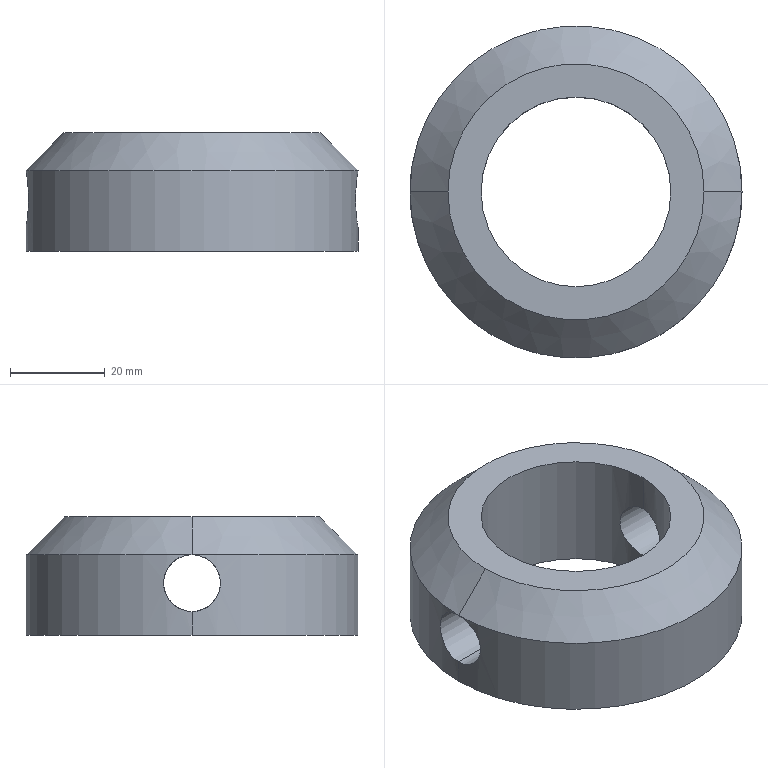Part | SolidWorks | features Chamfer 1, Extrusion 1, ICE 1 | 1 solid | 12 faces | box 70 x 70 x 25 mm | volume 54879 mm3 | cylinder 8 | cone 2 | plane 2 | commonest cylinder face diameters 12 x4 40 x2 70 x2
STEP:
#1=CARTESIAN_POINT('',(-35.,0.,17.));
#2=VERTEX_POINT('',#1);
#3=CARTESIAN_POINT('',(-35.,0.,5.));
#4=VERTEX_POINT('',#3);
#5=CARTESIAN_POINT('',(-35.,0.,17.));
#6=CARTESIAN_POINT('',(-35.,-0.3971,17.));
#7=CARTESIAN_POINT('',(-34.993,-0.7875,16.961));
#8=CARTESIAN_POINT('',(-34.974,-1.363,16.846));
#9=CARTESIAN_POINT('',(-34.966,-1.554,16.799));
#10=CARTESIAN_POINT('',(-34.947,-1.931,16.684));
#11=CARTESIAN_POINT('',(-34.936,-2.118,16.617));
#12=CARTESIAN_POINT('',(-34.9,-2.663,16.391));
#13=CARTESIAN_POINT('',(-34.872,-3.007,16.207));
#14=CARTESIAN_POINT('',(-34.81,-3.659,15.772));
#15=CARTESIAN_POINT('',(-34.776,-3.967,15.519));
#16=CARTESIAN_POINT('',(-34.708,-4.519,14.966));
#17=CARTESIAN_POINT('',(-34.675,-4.767,14.665));
#18=CARTESIAN_POINT('',(-34.611,-5.206,14.009));
#19=CARTESIAN_POINT('',(-34.583,-5.392,13.661));
#20=CARTESIAN_POINT('',(-34.547,-5.616,13.12));
#21=CARTESIAN_POINT('',(-34.536,-5.682,12.936));
#22=CARTESIAN_POINT('',(-34.517,-5.797,12.56));
#23=CARTESIAN_POINT('',(-34.508,-5.845,12.367));
#24=CARTESIAN_POINT('',(-34.489,-5.961,11.786));
#25=CARTESIAN_POINT('',(-34.482,-6.,11.397));
#26=CARTESIAN_POINT('',(-34.482,-6.,10.613));
#27=CARTESIAN_POINT('',(-34.489,-5.961,10.214));
#28=CARTESIAN_POINT('',(-34.515,-5.808,9.444));
#29=CARTESIAN_POINT('',(-34.534,-5.695,9.07));
#30=CARTESIAN_POINT('',(-34.57,-5.469,8.524));
#31=CARTESIAN_POINT('',(-34.584,-5.384,8.345));
#32=CARTESIAN_POINT('',(-34.612,-5.199,7.998));
#33=CARTESIAN_POINT('',(-34.627,-5.098,7.83));
#34=CARTESIAN_POINT('',(-34.674,-4.773,7.343));
#35=CARTESIAN_POINT('',(-34.707,-4.524,7.039));
#36=CARTESIAN_POINT('',(-34.776,-3.966,6.48));
#37=CARTESIAN_POINT('',(-34.809,-3.664,6.233));
#38=CARTESIAN_POINT('',(-34.856,-3.177,5.907));
#39=CARTESIAN_POINT('',(-34.871,-3.01,5.806));
#40=CARTESIAN_POINT('',(-34.899,-2.662,5.619));
#41=CARTESIAN_POINT('',(-34.912,-2.483,5.534));
#42=CARTESIAN_POINT('',(-34.948,-1.939,5.308));
#43=CARTESIAN_POINT('',(-34.967,-1.565,5.194));
#44=CARTESIAN_POINT('',(-34.993,-0.7947,5.04));
#45=CARTESIAN_POINT('',(-35.,-0.3971,5.));
#46=CARTESIAN_POINT('',(-35.,0.,5.));
#47=B_SPLINE_CURVE_WITH_KNOTS('',3,(#5,#6,#7,#8,#9,#10,#11,#12,#13,#14,#15,#16,#17,#18,#19,#20,#21,#22,#23,#24,#25,#26,#27,#28,#29,#30,#31,#32,#33,#34,#35,#36,#37,#38,#39,#40,#41,#42,#43,#44,#45,#46),.UNSPECIFIED.,.F.,.F.,(4,2,2,2,2,2,2,2,2,2,2,2,2,2,2,2,2,2,2,2,4),(0.01879,0.01996,0.02055,0.02114,0.02231,0.02349,0.02466,0.02583,0.02642,0.02701,0.02818,0.02936,0.03053,0.03112,0.03171,0.03288,0.03405,0.03464,0.03523,0.0364,0.03758),.UNSPECIFIED.);
#48=EDGE_CURVE('',#2,#4,#47,.T.);
#49=ORIENTED_EDGE('',*,*,#48,.F.);
#50=CARTESIAN_POINT('',(-20.,0.,17.));
#51=VERTEX_POINT('',#50);
#52=CARTESIAN_POINT('',(-35.,0.,17.));
#53=DIRECTION('',(1.,0.,0.));
#54=VECTOR('',#53,1000.);
#55=LINE('',#52,#54);
#56=EDGE_CURVE('',#2,#51,#55,.T.);
#57=ORIENTED_EDGE('',*,*,#56,.T.);
#58=CARTESIAN_POINT('',(-20.,0.,5.));
#59=VERTEX_POINT('',#58);
#60=CARTESIAN_POINT('',(-20.,0.,17.));
#61=CARTESIAN_POINT('',(-20.,-0.3989,17.));
#62=CARTESIAN_POINT('',(-19.988,-0.7907,16.961));
#63=CARTESIAN_POINT('',(-19.954,-1.368,16.845));
#64=CARTESIAN_POINT('',(-19.94,-1.559,16.797));
#65=CARTESIAN_POINT('',(-19.907,-1.937,16.682));
#66=CARTESIAN_POINT('',(-19.888,-2.125,16.615));
#67=CARTESIAN_POINT('',(-19.824,-2.669,16.388));
#68=CARTESIAN_POINT('',(-19.775,-3.013,16.204));
#69=CARTESIAN_POINT('',(-19.692,-3.501,15.877));
#70=CARTESIAN_POINT('',(-19.663,-3.659,15.759));
#71=CARTESIAN_POINT('',(-19.604,-3.962,15.51));
#72=CARTESIAN_POINT('',(-19.574,-4.107,15.379));
#73=CARTESIAN_POINT('',(-19.485,-4.519,14.966));
#74=CARTESIAN_POINT('',(-19.425,-4.767,14.665));
#75=CARTESIAN_POINT('',(-19.312,-5.205,14.01));
#76=CARTESIAN_POINT('',(-19.261,-5.39,13.665));
#77=CARTESIAN_POINT('',(-19.196,-5.615,13.124));
#78=CARTESIAN_POINT('',(-19.176,-5.681,12.94));
#79=CARTESIAN_POINT('',(-19.142,-5.796,12.563));
#80=CARTESIAN_POINT('',(-19.127,-5.845,12.369));
#81=CARTESIAN_POINT('',(-19.091,-5.961,11.788));
#82=CARTESIAN_POINT('',(-19.079,-6.,11.397));
#83=CARTESIAN_POINT('',(-19.079,-6.,10.609));
#84=CARTESIAN_POINT('',(-19.091,-5.961,10.209));
#85=CARTESIAN_POINT('',(-19.139,-5.806,9.437));
#86=CARTESIAN_POINT('',(-19.174,-5.692,9.062));
#87=CARTESIAN_POINT('',(-19.261,-5.389,8.333));
#88=CARTESIAN_POINT('',(-19.313,-5.202,7.985));
#89=CARTESIAN_POINT('',(-19.397,-4.877,7.5));
#90=CARTESIAN_POINT('',(-19.425,-4.761,7.343));
#91=CARTESIAN_POINT('',(-19.485,-4.513,7.041));
#92=CARTESIAN_POINT('',(-19.515,-4.38,6.894));
#93=CARTESIAN_POINT('',(-19.605,-3.964,6.479));
#94=CARTESIAN_POINT('',(-19.664,-3.664,6.232));
#95=CARTESIAN_POINT('',(-19.774,-3.015,5.798));
#96=CARTESIAN_POINT('',(-19.825,-2.664,5.61));
#97=CARTESIAN_POINT('',(-19.909,-1.941,5.309));
#98=CARTESIAN_POINT('',(-19.942,-1.566,5.195));
#99=CARTESIAN_POINT('',(-19.977,-0.985,5.078));
#100=CARTESIAN_POINT('',(-19.985,-0.787,5.049));
#101=CARTESIAN_POINT('',(-19.997,-0.3932,5.01));
#102=CARTESIAN_POINT('',(-20.,-0.1965,5.));
#103=CARTESIAN_POINT('',(-20.,0.,5.));
#104=B_SPLINE_CURVE_WITH_KNOTS('',3,(#60,#61,#62,#63,#64,#65,#66,#67,#68,#69,#70,#71,#72,#73,#74,#75,#76,#77,#78,#79,#80,#81,#82,#83,#84,#85,#86,#87,#88,#89,#90,#91,#92,#93,#94,#95,#96,#97,#98,#99,#100,#101,#102,#103),.UNSPECIFIED.,.F.,.F.,(4,2,2,2,2,2,2,2,2,2,2,2,2,2,2,2,2,2,2,2,2,4),(0.,0.001179,0.001769,0.002359,0.003538,0.004127,0.004717,0.005896,0.007076,0.007665,0.008255,0.009434,0.01061,0.01179,0.01297,0.01356,0.01415,0.01533,0.01651,0.01769,0.01828,0.01887),.UNSPECIFIED.);
#105=EDGE_CURVE('',#51,#59,#104,.T.);
#106=ORIENTED_EDGE('',*,*,#105,.T.);
#107=CARTESIAN_POINT('',(-35.,0.,5.));
#108=DIRECTION('',(1.,0.,0.));
#109=VECTOR('',#108,1000.);
#110=LINE('',#107,#109);
#111=EDGE_CURVE('',#4,#59,#110,.T.);
#112=ORIENTED_EDGE('',*,*,#111,.F.);
#113=EDGE_LOOP('',(#49,#57,#106,#112));
#114=FACE_OUTER_BOUND('',#113,.T.);
#115=CARTESIAN_POINT('',(-35.,0.,11.));
#116=DIRECTION('',(1.,0.,0.));
#117=DIRECTION('',(0.,0.,-1.));
#118=AXIS2_PLACEMENT_3D('',#115,#116,#117);
#119=CYLINDRICAL_SURFACE('',#118,6.);
#120=ADVANCED_FACE('',(#114),#119,.F.);
#121=CARTESIAN_POINT('',(20.,0.,5.));
#122=VERTEX_POINT('',#121);
#123=CARTESIAN_POINT('',(20.,0.,17.));
#124=VERTEX_POINT('',#123);
#125=CARTESIAN_POINT('',(20.,0.,5.));
#126=CARTESIAN_POINT('',(20.,-0.3989,5.));
#127=CARTESIAN_POINT('',(19.988,-0.7907,5.039));
#128=CARTESIAN_POINT('',(19.954,-1.368,5.155));
#129=CARTESIAN_POINT('',(19.94,-1.559,5.203));
#130=CARTESIAN_POINT('',(19.907,-1.937,5.318));
#131=CARTESIAN_POINT('',(19.888,-2.125,5.385));
#132=CARTESIAN_POINT('',(19.824,-2.669,5.612));
#133=CARTESIAN_POINT('',(19.775,-3.013,5.796));
#134=CARTESIAN_POINT('',(19.692,-3.501,6.123));
#135=CARTESIAN_POINT('',(19.663,-3.659,6.241));
#136=CARTESIAN_POINT('',(19.604,-3.962,6.49));
#137=CARTESIAN_POINT('',(19.574,-4.107,6.621));
#138=CARTESIAN_POINT('',(19.485,-4.519,7.034));
#139=CARTESIAN_POINT('',(19.425,-4.767,7.335));
#140=CARTESIAN_POINT('',(19.312,-5.205,7.99));
#141=CARTESIAN_POINT('',(19.261,-5.39,8.335));
#142=CARTESIAN_POINT('',(19.196,-5.615,8.876));
#143=CARTESIAN_POINT('',(19.176,-5.681,9.06));
#144=CARTESIAN_POINT('',(19.142,-5.796,9.437));
#145=CARTESIAN_POINT('',(19.127,-5.845,9.631));
#146=CARTESIAN_POINT('',(19.091,-5.961,10.212));
#147=CARTESIAN_POINT('',(19.079,-6.,10.603));
#148=CARTESIAN_POINT('',(19.079,-6.,11.391));
#149=CARTESIAN_POINT('',(19.091,-5.961,11.791));
#150=CARTESIAN_POINT('',(19.139,-5.806,12.563));
#151=CARTESIAN_POINT('',(19.174,-5.692,12.938));
#152=CARTESIAN_POINT('',(19.261,-5.389,13.667));
#153=CARTESIAN_POINT('',(19.313,-5.202,14.015));
#154=CARTESIAN_POINT('',(19.397,-4.877,14.5));
#155=CARTESIAN_POINT('',(19.425,-4.761,14.657));
#156=CARTESIAN_POINT('',(19.485,-4.513,14.959));
#157=CARTESIAN_POINT('',(19.515,-4.38,15.106));
#158=CARTESIAN_POINT('',(19.605,-3.964,15.521));
#159=CARTESIAN_POINT('',(19.664,-3.664,15.768));
#160=CARTESIAN_POINT('',(19.774,-3.015,16.202));
#161=CARTESIAN_POINT('',(19.825,-2.664,16.39));
#162=CARTESIAN_POINT('',(19.909,-1.941,16.691));
#163=CARTESIAN_POINT('',(19.942,-1.566,16.805));
#164=CARTESIAN_POINT('',(19.977,-0.985,16.922));
#165=CARTESIAN_POINT('',(19.985,-0.787,16.951));
#166=CARTESIAN_POINT('',(19.997,-0.3932,16.99));
#167=CARTESIAN_POINT('',(20.,-0.1965,17.));
#168=CARTESIAN_POINT('',(20.,0.,17.));
#169=B_SPLINE_CURVE_WITH_KNOTS('',3,(#125,#126,#127,#128,#129,#130,#131,#132,#133,#134,#135,#136,#137,#138,#139,#140,#141,#142,#143,#144,#145,#146,#147,#148,#149,#150,#151,#152,#153,#154,#155,#156,#157,#158,#159,#160,#161,#162,#163,#164,#165,#166,#167,#168),.UNSPECIFIED.,.F.,.F.,(4,2,2,2,2,2,2,2,2,2,2,2,2,2,2,2,2,2,2,2,2,4),(0.,0.001179,0.001769,0.002359,0.003538,0.004127,0.004717,0.005896,0.007076,0.007665,0.008255,0.009434,0.01061,0.01179,0.01297,0.01356,0.01415,0.01533,0.01651,0.01769,0.01828,0.01887),.UNSPECIFIED.);
#170=EDGE_CURVE('',#122,#124,#169,.T.);
#171=ORIENTED_EDGE('',*,*,#170,.T.);
#172=CARTESIAN_POINT('',(35.,0.,17.));
#173=VERTEX_POINT('',#172);
#174=CARTESIAN_POINT('',(-35.,0.,17.));
#175=DIRECTION('',(1.,0.,0.));
#176=VECTOR('',#175,1000.);
#177=LINE('',#174,#176);
#178=EDGE_CURVE('',#124,#173,#177,.T.);
#179=ORIENTED_EDGE('',*,*,#178,.T.);
#180=CARTESIAN_POINT('',(35.,0.,5.));
#181=VERTEX_POINT('',#180);
#182=CARTESIAN_POINT('',(35.,0.,5.));
#183=CARTESIAN_POINT('',(35.,-0.3972,5.));
#184=CARTESIAN_POINT('',(34.993,-0.7877,5.039));
#185=CARTESIAN_POINT('',(34.974,-1.364,5.154));
#186=CARTESIAN_POINT('',(34.966,-1.554,5.201));
#187=CARTESIAN_POINT('',(34.947,-1.931,5.316));
#188=CARTESIAN_POINT('',(34.936,-2.119,5.383));
#189=CARTESIAN_POINT('',(34.9,-2.663,5.609));
#190=CARTESIAN_POINT('',(34.872,-3.008,5.794));
#191=CARTESIAN_POINT('',(34.81,-3.659,6.229));
#192=CARTESIAN_POINT('',(34.776,-3.967,6.482));
#193=CARTESIAN_POINT('',(34.708,-4.52,7.035));
#194=CARTESIAN_POINT('',(34.674,-4.768,7.336));
#195=CARTESIAN_POINT('',(34.611,-5.206,7.992));
#196=CARTESIAN_POINT('',(34.582,-5.392,8.34));
#197=CARTESIAN_POINT('',(34.546,-5.617,8.881));
#198=CARTESIAN_POINT('',(34.536,-5.683,9.066));
#199=CARTESIAN_POINT('',(34.517,-5.797,9.442));
#200=CARTESIAN_POINT('',(34.508,-5.846,9.635));
#201=CARTESIAN_POINT('',(34.489,-5.962,10.216));
#202=CARTESIAN_POINT('',(34.482,-6.,10.606));
#203=CARTESIAN_POINT('',(34.482,-6.,11.39));
#204=CARTESIAN_POINT('',(34.489,-5.961,11.788));
#205=CARTESIAN_POINT('',(34.515,-5.807,12.558));
#206=CARTESIAN_POINT('',(34.534,-5.694,12.933));
#207=CARTESIAN_POINT('',(34.57,-5.468,13.478));
#208=CARTESIAN_POINT('',(34.584,-5.383,13.658));
#209=CARTESIAN_POINT('',(34.612,-5.197,14.005));
#210=CARTESIAN_POINT('',(34.627,-5.096,14.173));
#211=CARTESIAN_POINT('',(34.674,-4.771,14.66));
#212=CARTESIAN_POINT('',(34.708,-4.522,14.963));
#213=CARTESIAN_POINT('',(34.776,-3.963,15.522));
#214=CARTESIAN_POINT('',(34.81,-3.661,15.77));
#215=CARTESIAN_POINT('',(34.856,-3.174,16.095));
#216=CARTESIAN_POINT('',(34.871,-3.006,16.196));
#217=CARTESIAN_POINT('',(34.899,-2.659,16.382));
#218=CARTESIAN_POINT('',(34.913,-2.479,16.467));
#219=CARTESIAN_POINT('',(34.948,-1.935,16.693));
#220=CARTESIAN_POINT('',(34.967,-1.561,16.807));
#221=CARTESIAN_POINT('',(34.993,-0.7902,16.961));
#222=CARTESIAN_POINT('',(35.,-0.392,17.));
#223=CARTESIAN_POINT('',(35.,0.,17.));
#224=B_SPLINE_CURVE_WITH_KNOTS('',3,(#182,#183,#184,#185,#186,#187,#188,#189,#190,#191,#192,#193,#194,#195,#196,#197,#198,#199,#200,#201,#202,#203,#204,#205,#206,#207,#208,#209,#210,#211,#212,#213,#214,#215,#216,#217,#218,#219,#220,#221,#222,#223),.UNSPECIFIED.,.F.,.F.,(4,2,2,2,2,2,2,2,2,2,2,2,2,2,2,2,2,2,2,2,4),(0.,0.001175,0.001762,0.002349,0.003524,0.004698,0.005873,0.007048,0.007635,0.008222,0.009397,0.01057,0.01175,0.01233,0.01292,0.0141,0.01527,0.01586,0.01644,0.01762,0.01879),.UNSPECIFIED.);
#225=EDGE_CURVE('',#181,#173,#224,.T.);
#226=ORIENTED_EDGE('',*,*,#225,.F.);
#227=CARTESIAN_POINT('',(-35.,0.,5.));
#228=DIRECTION('',(1.,0.,0.));
#229=VECTOR('',#228,1000.);
#230=LINE('',#227,#229);
#231=EDGE_CURVE('',#122,#181,#230,.T.);
#232=ORIENTED_EDGE('',*,*,#231,.F.);
#233=EDGE_LOOP('',(#171,#179,#226,#232));
#234=FACE_OUTER_BOUND('',#233,.T.);
#235=CARTESIAN_POINT('',(-35.,0.,11.));
#236=DIRECTION('',(1.,0.,0.));
#237=DIRECTION('',(0.,0.,-1.));
#238=AXIS2_PLACEMENT_3D('',#235,#236,#237);
#239=CYLINDRICAL_SURFACE('',#238,6.);
#240=ADVANCED_FACE('',(#234),#239,.F.);
#241=CARTESIAN_POINT('',(27.,0.,25.));
#242=VERTEX_POINT('',#241);
#243=CARTESIAN_POINT('',(-27.,0.,25.));
#244=VERTEX_POINT('',#243);
#245=CARTESIAN_POINT('',(0.,0.,25.));
#246=DIRECTION('',(0.,0.,1.));
#247=DIRECTION('',(1.,0.,0.));
#248=AXIS2_PLACEMENT_3D('',#245,#246,#247);
#249=CIRCLE('',#248,27.);
#250=EDGE_CURVE('',#242,#244,#249,.T.);
#251=ORIENTED_EDGE('',*,*,#250,.F.);
#252=CARTESIAN_POINT('',(27.,0.,25.));
#253=DIRECTION('',(0.7071,0.,-0.7071));
#254=VECTOR('',#253,1000.);
#255=LINE('',#252,#254);
#256=EDGE_CURVE('',#242,#173,#255,.T.);
#257=ORIENTED_EDGE('',*,*,#256,.T.);
#258=CARTESIAN_POINT('',(0.,0.,17.));
#259=DIRECTION('',(0.,0.,-1.));
#260=DIRECTION('',(1.,0.,0.));
#261=AXIS2_PLACEMENT_3D('',#258,#259,#260);
#262=CIRCLE('',#261,35.);
#263=EDGE_CURVE('',#2,#173,#262,.T.);
#264=ORIENTED_EDGE('',*,*,#263,.F.);
#265=CARTESIAN_POINT('',(-27.,0.,25.));
#266=DIRECTION('',(-0.7071,0.,-0.7071));
#267=VECTOR('',#266,1000.);
#268=LINE('',#265,#267);
#269=EDGE_CURVE('',#244,#2,#268,.T.);
#270=ORIENTED_EDGE('',*,*,#269,.F.);
#271=EDGE_LOOP('',(#251,#257,#264,#270));
#272=FACE_OUTER_BOUND('',#271,.T.);
#273=CARTESIAN_POINT('',(0.,0.,25.));
#274=DIRECTION('',(0.,0.,-1.));
#275=DIRECTION('',(-1.,0.,0.));
#276=AXIS2_PLACEMENT_3D('',#273,#274,#275);
#277=CONICAL_SURFACE('',#276,27.,0.7854);
#278=ADVANCED_FACE('',(#272),#277,.T.);
#279=CARTESIAN_POINT('',(-20.,0.,25.));
#280=VERTEX_POINT('',#279);
#281=CARTESIAN_POINT('',(20.,0.,25.));
#282=VERTEX_POINT('',#281);
#283=CARTESIAN_POINT('',(0.,0.,25.));
#284=DIRECTION('',(0.,0.,1.));
#285=DIRECTION('',(1.,0.,0.));
#286=AXIS2_PLACEMENT_3D('',#283,#284,#285);
#287=CIRCLE('',#286,20.);
#288=EDGE_CURVE('',#280,#282,#287,.T.);
#289=ORIENTED_EDGE('',*,*,#288,.T.);
#290=CARTESIAN_POINT('',(20.,0.,25.));
#291=DIRECTION('',(0.,0.,-1.));
#292=VECTOR('',#291,1000.);
#293=LINE('',#290,#292);
#294=EDGE_CURVE('',#282,#124,#293,.T.);
#295=ORIENTED_EDGE('',*,*,#294,.T.);
#296=ORIENTED_EDGE('',*,*,#170,.F.);
#297=CARTESIAN_POINT('',(20.,0.,0.));
#298=VERTEX_POINT('',#297);
#299=CARTESIAN_POINT('',(20.,0.,25.));
#300=DIRECTION('',(0.,0.,-1.));
#301=VECTOR('',#300,1000.);
#302=LINE('',#299,#301);
#303=EDGE_CURVE('',#122,#298,#302,.T.);
#304=ORIENTED_EDGE('',*,*,#303,.T.);
#305=CARTESIAN_POINT('',(-20.,0.,0.));
#306=VERTEX_POINT('',#305);
#307=CARTESIAN_POINT('',(0.,0.,0.));
#308=DIRECTION('',(0.,0.,1.));
#309=DIRECTION('',(1.,0.,0.));
#310=AXIS2_PLACEMENT_3D('',#307,#308,#309);
#311=CIRCLE('',#310,20.);
#312=EDGE_CURVE('',#306,#298,#311,.T.);
#313=ORIENTED_EDGE('',*,*,#312,.F.);
#314=CARTESIAN_POINT('',(-20.,0.,25.));
#315=DIRECTION('',(0.,0.,-1.));
#316=VECTOR('',#315,1000.);
#317=LINE('',#314,#316);
#318=EDGE_CURVE('',#59,#306,#317,.T.);
#319=ORIENTED_EDGE('',*,*,#318,.F.);
#320=ORIENTED_EDGE('',*,*,#105,.F.);
#321=CARTESIAN_POINT('',(-20.,0.,25.));
#322=DIRECTION('',(0.,0.,-1.));
#323=VECTOR('',#322,1000.);
#324=LINE('',#321,#323);
#325=EDGE_CURVE('',#280,#51,#324,.T.);
#326=ORIENTED_EDGE('',*,*,#325,.F.);
#327=EDGE_LOOP('',(#289,#295,#296,#304,#313,#319,#320,#326));
#328=FACE_OUTER_BOUND('',#327,.T.);
#329=CARTESIAN_POINT('',(0.,0.,25.));
#330=DIRECTION('',(0.,0.,-1.));
#331=DIRECTION('',(-1.,0.,0.));
#332=AXIS2_PLACEMENT_3D('',#329,#330,#331);
#333=CYLINDRICAL_SURFACE('',#332,20.);
#334=ADVANCED_FACE('',(#328),#333,.F.);
#335=CARTESIAN_POINT('',(35.,0.,17.));
#336=CARTESIAN_POINT('',(35.,0.3919,17.));
#337=CARTESIAN_POINT('',(34.993,0.7819,16.962));
#338=CARTESIAN_POINT('',(34.967,1.558,16.808));
#339=CARTESIAN_POINT('',(34.948,1.936,16.693));
#340=CARTESIAN_POINT('',(34.913,2.477,16.468));
#341=CARTESIAN_POINT('',(34.9,2.654,16.385));
#342=CARTESIAN_POINT('',(34.872,3.001,16.199));
#343=CARTESIAN_POINT('',(34.856,3.171,16.097));
#344=CARTESIAN_POINT('',(34.809,3.662,15.769));
#345=CARTESIAN_POINT('',(34.776,3.963,15.522));
#346=CARTESIAN_POINT('',(34.708,4.517,14.969));
#347=CARTESIAN_POINT('',(34.674,4.77,14.661));
#348=CARTESIAN_POINT('',(34.612,5.205,14.011));
#349=CARTESIAN_POINT('',(34.583,5.389,13.667));
#350=CARTESIAN_POINT('',(34.547,5.616,13.121));
#351=CARTESIAN_POINT('',(34.536,5.683,12.934));
#352=CARTESIAN_POINT('',(34.517,5.798,12.557));
#353=CARTESIAN_POINT('',(34.508,5.845,12.367));
#354=CARTESIAN_POINT('',(34.489,5.96,11.792));
#355=CARTESIAN_POINT('',(34.482,6.,11.4));
#356=CARTESIAN_POINT('',(34.482,6.,10.607));
#357=CARTESIAN_POINT('',(34.489,5.962,10.217));
#358=CARTESIAN_POINT('',(34.508,5.847,9.641));
#359=CARTESIAN_POINT('',(34.516,5.8,9.45));
#360=CARTESIAN_POINT('',(34.535,5.685,9.072));
#361=CARTESIAN_POINT('',(34.546,5.618,8.885));
#362=CARTESIAN_POINT('',(34.582,5.393,8.341));
#363=CARTESIAN_POINT('',(34.611,5.209,7.997));
#364=CARTESIAN_POINT('',(34.658,4.882,7.507));
#365=CARTESIAN_POINT('',(34.674,4.764,7.348));
#366=CARTESIAN_POINT('',(34.708,4.515,7.043));
#367=CARTESIAN_POINT('',(34.725,4.383,6.898));
#368=CARTESIAN_POINT('',(34.775,3.97,6.484));
#369=CARTESIAN_POINT('',(34.809,3.668,6.235));
#370=CARTESIAN_POINT('',(34.872,3.012,5.795));
#371=CARTESIAN_POINT('',(34.9,2.665,5.61));
#372=CARTESIAN_POINT('',(34.936,2.124,5.385));
#373=CARTESIAN_POINT('',(34.947,1.94,5.319));
#374=CARTESIAN_POINT('',(34.966,1.564,5.204));
#375=CARTESIAN_POINT('',(34.974,1.371,5.155));
#376=CARTESIAN_POINT('',(34.993,0.7894,5.039));
#377=CARTESIAN_POINT('',(35.,0.3971,5.));
#378=CARTESIAN_POINT('',(35.,0.,5.));
#379=B_SPLINE_CURVE_WITH_KNOTS('',3,(#335,#336,#337,#338,#339,#340,#341,#342,#343,#344,#345,#346,#347,#348,#349,#350,#351,#352,#353,#354,#355,#356,#357,#358,#359,#360,#361,#362,#363,#364,#365,#366,#367,#368,#369,#370,#371,#372,#373,#374,#375,#376,#377,#378),.UNSPECIFIED.,.F.,.F.,(4,2,2,2,2,2,2,2,2,2,2,2,2,2,2,2,2,2,2,2,2,4),(0.01879,0.01997,0.02114,0.02173,0.02232,0.02349,0.02466,0.02584,0.02643,0.02701,0.02819,0.02936,0.02995,0.03054,0.03171,0.0323,0.03289,0.03406,0.03523,0.03582,0.03641,0.03758),.UNSPECIFIED.);
#380=EDGE_CURVE('',#173,#181,#379,.T.);
#381=ORIENTED_EDGE('',*,*,#380,.T.);
#382=CARTESIAN_POINT('',(35.,0.,0.));
#383=VERTEX_POINT('',#382);
#384=CARTESIAN_POINT('',(35.,0.,25.));
#385=DIRECTION('',(0.,0.,-1.));
#386=VECTOR('',#385,1000.);
#387=LINE('',#384,#386);
#388=EDGE_CURVE('',#181,#383,#387,.T.);
#389=ORIENTED_EDGE('',*,*,#388,.T.);
#390=CARTESIAN_POINT('',(-35.,0.,0.));
#391=VERTEX_POINT('',#390);
#392=CARTESIAN_POINT('',(0.,0.,0.));
#393=DIRECTION('',(0.,0.,1.));
#394=DIRECTION('',(1.,0.,0.));
#395=AXIS2_PLACEMENT_3D('',#392,#393,#394);
#396=CIRCLE('',#395,35.);
#397=EDGE_CURVE('',#383,#391,#396,.T.);
#398=ORIENTED_EDGE('',*,*,#397,.T.);
#399=CARTESIAN_POINT('',(-35.,0.,25.));
#400=DIRECTION('',(0.,0.,-1.));
#401=VECTOR('',#400,1000.);
#402=LINE('',#399,#401);
#403=EDGE_CURVE('',#4,#391,#402,.T.);
#404=ORIENTED_EDGE('',*,*,#403,.F.);
#405=CARTESIAN_POINT('',(-35.,0.,5.));
#406=CARTESIAN_POINT('',(-35.,0.3971,5.));
#407=CARTESIAN_POINT('',(-34.993,0.7875,5.039));
#408=CARTESIAN_POINT('',(-34.974,1.363,5.154));
#409=CARTESIAN_POINT('',(-34.966,1.554,5.201));
#410=CARTESIAN_POINT('',(-34.947,1.931,5.316));
#411=CARTESIAN_POINT('',(-34.936,2.118,5.383));
#412=CARTESIAN_POINT('',(-34.9,2.663,5.609));
#413=CARTESIAN_POINT('',(-34.872,3.007,5.793));
#414=CARTESIAN_POINT('',(-34.81,3.659,6.228));
#415=CARTESIAN_POINT('',(-34.776,3.967,6.481));
#416=CARTESIAN_POINT('',(-34.708,4.519,7.034));
#417=CARTESIAN_POINT('',(-34.675,4.767,7.335));
#418=CARTESIAN_POINT('',(-34.611,5.206,7.991));
#419=CARTESIAN_POINT('',(-34.583,5.392,8.339));
#420=CARTESIAN_POINT('',(-34.547,5.616,8.88));
#421=CARTESIAN_POINT('',(-34.536,5.682,9.064));
#422=CARTESIAN_POINT('',(-34.517,5.797,9.44));
#423=CARTESIAN_POINT('',(-34.508,5.845,9.633));
#424=CARTESIAN_POINT('',(-34.489,5.961,10.214));
#425=CARTESIAN_POINT('',(-34.482,6.,10.603));
#426=CARTESIAN_POINT('',(-34.482,6.,11.387));
#427=CARTESIAN_POINT('',(-34.489,5.961,11.786));
#428=CARTESIAN_POINT('',(-34.515,5.808,12.556));
#429=CARTESIAN_POINT('',(-34.534,5.695,12.93));
#430=CARTESIAN_POINT('',(-34.57,5.469,13.476));
#431=CARTESIAN_POINT('',(-34.584,5.384,13.655));
#432=CARTESIAN_POINT('',(-34.612,5.199,14.002));
#433=CARTESIAN_POINT('',(-34.627,5.098,14.17));
#434=CARTESIAN_POINT('',(-34.674,4.773,14.657));
#435=CARTESIAN_POINT('',(-34.707,4.524,14.961));
#436=CARTESIAN_POINT('',(-34.776,3.966,15.52));
#437=CARTESIAN_POINT('',(-34.809,3.664,15.767));
#438=CARTESIAN_POINT('',(-34.856,3.177,16.093));
#439=CARTESIAN_POINT('',(-34.871,3.01,16.194));
#440=CARTESIAN_POINT('',(-34.899,2.662,16.381));
#441=CARTESIAN_POINT('',(-34.912,2.483,16.466));
#442=CARTESIAN_POINT('',(-34.948,1.939,16.692));
#443=CARTESIAN_POINT('',(-34.967,1.565,16.806));
#444=CARTESIAN_POINT('',(-34.993,0.7947,16.96));
#445=CARTESIAN_POINT('',(-35.,0.3971,17.));
#446=CARTESIAN_POINT('',(-35.,0.,17.));
#447=B_SPLINE_CURVE_WITH_KNOTS('',3,(#405,#406,#407,#408,#409,#410,#411,#412,#413,#414,#415,#416,#417,#418,#419,#420,#421,#422,#423,#424,#425,#426,#427,#428,#429,#430,#431,#432,#433,#434,#435,#436,#437,#438,#439,#440,#441,#442,#443,#444,#445,#446),.UNSPECIFIED.,.F.,.F.,(4,2,2,2,2,2,2,2,2,2,2,2,2,2,2,2,2,2,2,2,4),(0.,0.001174,0.001761,0.002349,0.003523,0.004697,0.005871,0.007046,0.007633,0.00822,0.009394,0.01057,0.01174,0.01233,0.01292,0.01409,0.01527,0.01585,0.01644,0.01761,0.01879),.UNSPECIFIED.);
#448=EDGE_CURVE('',#4,#2,#447,.T.);
#449=ORIENTED_EDGE('',*,*,#448,.T.);
#450=ORIENTED_EDGE('',*,*,#263,.T.);
#451=EDGE_LOOP('',(#381,#389,#398,#404,#449,#450));
#452=FACE_OUTER_BOUND('',#451,.T.);
#453=CARTESIAN_POINT('',(0.,0.,25.));
#454=DIRECTION('',(0.,0.,-1.));
#455=DIRECTION('',(-1.,0.,0.));
#456=AXIS2_PLACEMENT_3D('',#453,#454,#455);
#457=CYLINDRICAL_SURFACE('',#456,35.);
#458=ADVANCED_FACE('',(#452),#457,.T.);
#459=CARTESIAN_POINT('',(0.,0.,25.));
#460=DIRECTION('',(0.,0.,1.));
#461=DIRECTION('',(1.,0.,0.));
#462=AXIS2_PLACEMENT_3D('',#459,#460,#461);
#463=CIRCLE('',#462,27.);
#464=EDGE_CURVE('',#244,#242,#463,.T.);
#465=ORIENTED_EDGE('',*,*,#464,.T.);
#466=ORIENTED_EDGE('',*,*,#250,.T.);
#467=EDGE_LOOP('',(#465,#466));
#468=FACE_OUTER_BOUND('',#467,.T.);
#469=ORIENTED_EDGE('',*,*,#288,.F.);
#470=CARTESIAN_POINT('',(0.,0.,25.));
#471=DIRECTION('',(0.,0.,1.));
#472=DIRECTION('',(1.,0.,0.));
#473=AXIS2_PLACEMENT_3D('',#470,#471,#472);
#474=CIRCLE('',#473,20.);
#475=EDGE_CURVE('',#282,#280,#474,.T.);
#476=ORIENTED_EDGE('',*,*,#475,.F.);
#477=EDGE_LOOP('',(#469,#476));
#478=FACE_BOUND('',#477,.T.);
#479=CARTESIAN_POINT('',(0.,0.,25.));
#480=DIRECTION('',(0.,0.,1.));
#481=DIRECTION('',(1.,0.,0.));
#482=AXIS2_PLACEMENT_3D('',#479,#480,#481);
#483=PLANE('',#482);
#484=ADVANCED_FACE('',(#468,#478),#483,.T.);
#485=CARTESIAN_POINT('',(0.,0.,0.));
#486=DIRECTION('',(0.,0.,1.));
#487=DIRECTION('',(1.,0.,0.));
#488=AXIS2_PLACEMENT_3D('',#485,#486,#487);
#489=CIRCLE('',#488,35.);
#490=EDGE_CURVE('',#391,#383,#489,.T.);
#491=ORIENTED_EDGE('',*,*,#490,.F.);
#492=ORIENTED_EDGE('',*,*,#397,.F.);
#493=EDGE_LOOP('',(#491,#492));
#494=FACE_OUTER_BOUND('',#493,.T.);
#495=ORIENTED_EDGE('',*,*,#312,.T.);
#496=CARTESIAN_POINT('',(0.,0.,0.));
#497=DIRECTION('',(0.,0.,1.));
#498=DIRECTION('',(1.,0.,0.));
#499=AXIS2_PLACEMENT_3D('',#496,#497,#498);
#500=CIRCLE('',#499,20.);
#501=EDGE_CURVE('',#298,#306,#500,.T.);
#502=ORIENTED_EDGE('',*,*,#501,.T.);
#503=EDGE_LOOP('',(#495,#502));
#504=FACE_BOUND('',#503,.T.);
#505=CARTESIAN_POINT('',(0.,0.,0.));
#506=DIRECTION('',(0.,0.,1.));
#507=DIRECTION('',(1.,0.,0.));
#508=AXIS2_PLACEMENT_3D('',#505,#506,#507);
#509=PLANE('',#508);
#510=ADVANCED_FACE('',(#494,#504),#509,.F.);
#511=ORIENTED_EDGE('',*,*,#388,.F.);
#512=ORIENTED_EDGE('',*,*,#225,.T.);
#513=CARTESIAN_POINT('',(0.,0.,17.));
#514=DIRECTION('',(0.,0.,-1.));
#515=DIRECTION('',(1.,0.,0.));
#516=AXIS2_PLACEMENT_3D('',#513,#514,#515);
#517=CIRCLE('',#516,35.);
#518=EDGE_CURVE('',#173,#2,#517,.T.);
#519=ORIENTED_EDGE('',*,*,#518,.T.);
#520=ORIENTED_EDGE('',*,*,#48,.T.);
#521=ORIENTED_EDGE('',*,*,#403,.T.);
#522=ORIENTED_EDGE('',*,*,#490,.T.);
#523=EDGE_LOOP('',(#511,#512,#519,#520,#521,#522));
#524=FACE_OUTER_BOUND('',#523,.T.);
#525=CARTESIAN_POINT('',(0.,0.,25.));
#526=DIRECTION('',(0.,0.,-1.));
#527=DIRECTION('',(-1.,0.,0.));
#528=AXIS2_PLACEMENT_3D('',#525,#526,#527);
#529=CYLINDRICAL_SURFACE('',#528,35.);
#530=ADVANCED_FACE('',(#524),#529,.T.);
#531=ORIENTED_EDGE('',*,*,#294,.F.);
#532=ORIENTED_EDGE('',*,*,#475,.T.);
#533=ORIENTED_EDGE('',*,*,#325,.T.);
#534=CARTESIAN_POINT('',(-20.,0.,5.));
#535=CARTESIAN_POINT('',(-20.,0.393,5.));
#536=CARTESIAN_POINT('',(-19.988,0.7871,5.039));
#537=CARTESIAN_POINT('',(-19.942,1.566,5.194));
#538=CARTESIAN_POINT('',(-19.909,1.941,5.309));
#539=CARTESIAN_POINT('',(-19.825,2.664,5.61));
#540=CARTESIAN_POINT('',(-19.774,3.016,5.798));
#541=CARTESIAN_POINT('',(-19.664,3.665,6.233));
#542=CARTESIAN_POINT('',(-19.605,3.965,6.48));
#543=CARTESIAN_POINT('',(-19.515,4.381,6.895));
#544=CARTESIAN_POINT('',(-19.484,4.513,7.042));
#545=CARTESIAN_POINT('',(-19.425,4.762,7.344));
#546=CARTESIAN_POINT('',(-19.396,4.878,7.501));
#547=CARTESIAN_POINT('',(-19.313,5.202,7.986));
#548=CARTESIAN_POINT('',(-19.261,5.388,8.33));
#549=CARTESIAN_POINT('',(-19.174,5.692,9.061));
#550=CARTESIAN_POINT('',(-19.139,5.806,9.436));
#551=CARTESIAN_POINT('',(-19.103,5.922,10.013));
#552=CARTESIAN_POINT('',(-19.094,5.951,10.208));
#553=CARTESIAN_POINT('',(-19.082,5.99,10.602));
#554=CARTESIAN_POINT('',(-19.079,6.,10.802));
#555=CARTESIAN_POINT('',(-19.079,6.,11.395));
#556=CARTESIAN_POINT('',(-19.091,5.961,11.786));
#557=CARTESIAN_POINT('',(-19.127,5.846,12.366));
#558=CARTESIAN_POINT('',(-19.141,5.797,12.559));
#559=CARTESIAN_POINT('',(-19.176,5.682,12.937));
#560=CARTESIAN_POINT('',(-19.196,5.616,13.122));
#561=CARTESIAN_POINT('',(-19.261,5.39,13.664));
#562=CARTESIAN_POINT('',(-19.312,5.206,14.009));
#563=CARTESIAN_POINT('',(-19.425,4.767,14.665));
#564=CARTESIAN_POINT('',(-19.485,4.519,14.966));
#565=CARTESIAN_POINT('',(-19.574,4.107,15.379));
#566=CARTESIAN_POINT('',(-19.604,3.963,15.51));
#567=CARTESIAN_POINT('',(-19.663,3.66,15.759));
#568=CARTESIAN_POINT('',(-19.692,3.501,15.877));
#569=CARTESIAN_POINT('',(-19.774,3.013,16.203));
#570=CARTESIAN_POINT('',(-19.824,2.67,16.388));
#571=CARTESIAN_POINT('',(-19.908,1.946,16.689));
#572=CARTESIAN_POINT('',(-19.943,1.563,16.806));
#573=CARTESIAN_POINT('',(-19.988,0.7911,16.961));
#574=CARTESIAN_POINT('',(-20.,0.3988,17.));
#575=CARTESIAN_POINT('',(-20.,0.,17.));
#576=B_SPLINE_CURVE_WITH_KNOTS('',3,(#534,#535,#536,#537,#538,#539,#540,#541,#542,#543,#544,#545,#546,#547,#548,#549,#550,#551,#552,#553,#554,#555,#556,#557,#558,#559,#560,#561,#562,#563,#564,#565,#566,#567,#568,#569,#570,#571,#572,#573,#574,#575),.UNSPECIFIED.,.F.,.F.,(4,2,2,2,2,2,2,2,2,2,2,2,2,2,2,2,2,2,2,2,4),(0.01887,0.02005,0.02123,0.0224,0.02358,0.02417,0.02476,0.02594,0.02712,0.02771,0.0283,0.02948,0.03007,0.03066,0.03184,0.03302,0.0336,0.03419,0.03537,0.03655,0.03773),.UNSPECIFIED.);
#577=EDGE_CURVE('',#59,#51,#576,.T.);
#578=ORIENTED_EDGE('',*,*,#577,.F.);
#579=ORIENTED_EDGE('',*,*,#318,.T.);
#580=ORIENTED_EDGE('',*,*,#501,.F.);
#581=ORIENTED_EDGE('',*,*,#303,.F.);
#582=CARTESIAN_POINT('',(20.,0.,17.));
#583=CARTESIAN_POINT('',(20.,0.393,17.));
#584=CARTESIAN_POINT('',(19.988,0.7871,16.961));
#585=CARTESIAN_POINT('',(19.942,1.566,16.806));
#586=CARTESIAN_POINT('',(19.909,1.941,16.691));
#587=CARTESIAN_POINT('',(19.825,2.664,16.39));
#588=CARTESIAN_POINT('',(19.774,3.016,16.202));
#589=CARTESIAN_POINT('',(19.664,3.665,15.767));
#590=CARTESIAN_POINT('',(19.605,3.965,15.52));
#591=CARTESIAN_POINT('',(19.515,4.381,15.105));
#592=CARTESIAN_POINT('',(19.484,4.513,14.958));
#593=CARTESIAN_POINT('',(19.425,4.762,14.656));
#594=CARTESIAN_POINT('',(19.396,4.878,14.499));
#595=CARTESIAN_POINT('',(19.313,5.202,14.014));
#596=CARTESIAN_POINT('',(19.261,5.388,13.67));
#597=CARTESIAN_POINT('',(19.174,5.692,12.939));
#598=CARTESIAN_POINT('',(19.139,5.806,12.564));
#599=CARTESIAN_POINT('',(19.103,5.922,11.987));
#600=CARTESIAN_POINT('',(19.094,5.951,11.792));
#601=CARTESIAN_POINT('',(19.082,5.99,11.398));
#602=CARTESIAN_POINT('',(19.079,6.,11.198));
#603=CARTESIAN_POINT('',(19.079,6.,10.605));
#604=CARTESIAN_POINT('',(19.091,5.961,10.214));
#605=CARTESIAN_POINT('',(19.127,5.846,9.634));
#606=CARTESIAN_POINT('',(19.141,5.797,9.441));
#607=CARTESIAN_POINT('',(19.176,5.682,9.063));
#608=CARTESIAN_POINT('',(19.196,5.616,8.878));
#609=CARTESIAN_POINT('',(19.261,5.39,8.336));
#610=CARTESIAN_POINT('',(19.312,5.206,7.991));
#611=CARTESIAN_POINT('',(19.425,4.767,7.335));
#612=CARTESIAN_POINT('',(19.485,4.519,7.034));
#613=CARTESIAN_POINT('',(19.574,4.107,6.621));
#614=CARTESIAN_POINT('',(19.604,3.963,6.49));
#615=CARTESIAN_POINT('',(19.663,3.66,6.241));
#616=CARTESIAN_POINT('',(19.692,3.501,6.123));
#617=CARTESIAN_POINT('',(19.774,3.013,5.797));
#618=CARTESIAN_POINT('',(19.824,2.67,5.612));
#619=CARTESIAN_POINT('',(19.908,1.946,5.311));
#620=CARTESIAN_POINT('',(19.943,1.563,5.194));
#621=CARTESIAN_POINT('',(19.988,0.7911,5.039));
#622=CARTESIAN_POINT('',(20.,0.3988,5.));
#623=CARTESIAN_POINT('',(20.,0.,5.));
#624=B_SPLINE_CURVE_WITH_KNOTS('',3,(#582,#583,#584,#585,#586,#587,#588,#589,#590,#591,#592,#593,#594,#595,#596,#597,#598,#599,#600,#601,#602,#603,#604,#605,#606,#607,#608,#609,#610,#611,#612,#613,#614,#615,#616,#617,#618,#619,#620,#621,#622,#623),.UNSPECIFIED.,.F.,.F.,(4,2,2,2,2,2,2,2,2,2,2,2,2,2,2,2,2,2,2,2,4),(0.01887,0.02005,0.02123,0.0224,0.02358,0.02417,0.02476,0.02594,0.02712,0.02771,0.0283,0.02948,0.03007,0.03066,0.03184,0.03302,0.0336,0.03419,0.03537,0.03655,0.03773),.UNSPECIFIED.);
#625=EDGE_CURVE('',#124,#122,#624,.T.);
#626=ORIENTED_EDGE('',*,*,#625,.F.);
#627=EDGE_LOOP('',(#531,#532,#533,#578,#579,#580,#581,#626));
#628=FACE_OUTER_BOUND('',#627,.T.);
#629=CARTESIAN_POINT('',(0.,0.,25.));
#630=DIRECTION('',(0.,0.,-1.));
#631=DIRECTION('',(-1.,0.,0.));
#632=AXIS2_PLACEMENT_3D('',#629,#630,#631);
#633=CYLINDRICAL_SURFACE('',#632,20.);
#634=ADVANCED_FACE('',(#628),#633,.F.);
#635=ORIENTED_EDGE('',*,*,#256,.F.);
#636=ORIENTED_EDGE('',*,*,#464,.F.);
#637=ORIENTED_EDGE('',*,*,#269,.T.);
#638=ORIENTED_EDGE('',*,*,#518,.F.);
#639=EDGE_LOOP('',(#635,#636,#637,#638));
#640=FACE_OUTER_BOUND('',#639,.T.);
#641=CARTESIAN_POINT('',(0.,0.,25.));
#642=DIRECTION('',(0.,0.,-1.));
#643=DIRECTION('',(-1.,0.,0.));
#644=AXIS2_PLACEMENT_3D('',#641,#642,#643);
#645=CONICAL_SURFACE('',#644,27.,0.7854);
#646=ADVANCED_FACE('',(#640),#645,.T.);
#647=ORIENTED_EDGE('',*,*,#178,.F.);
#648=ORIENTED_EDGE('',*,*,#625,.T.);
#649=ORIENTED_EDGE('',*,*,#231,.T.);
#650=ORIENTED_EDGE('',*,*,#380,.F.);
#651=EDGE_LOOP('',(#647,#648,#649,#650));
#652=FACE_OUTER_BOUND('',#651,.T.);
#653=CARTESIAN_POINT('',(-35.,0.,11.));
#654=DIRECTION('',(1.,0.,0.));
#655=DIRECTION('',(0.,0.,-1.));
#656=AXIS2_PLACEMENT_3D('',#653,#654,#655);
#657=CYLINDRICAL_SURFACE('',#656,6.);
#658=ADVANCED_FACE('',(#652),#657,.F.);
#659=ORIENTED_EDGE('',*,*,#56,.F.);
#660=ORIENTED_EDGE('',*,*,#448,.F.);
#661=ORIENTED_EDGE('',*,*,#111,.T.);
#662=ORIENTED_EDGE('',*,*,#577,.T.);
#663=EDGE_LOOP('',(#659,#660,#661,#662));
#664=FACE_OUTER_BOUND('',#663,.T.);
#665=CARTESIAN_POINT('',(-35.,0.,11.));
#666=DIRECTION('',(1.,0.,0.));
#667=DIRECTION('',(0.,0.,-1.));
#668=AXIS2_PLACEMENT_3D('',#665,#666,#667);
#669=CYLINDRICAL_SURFACE('',#668,6.);
#670=ADVANCED_FACE('',(#664),#669,.F.);
#671=CLOSED_SHELL('',(#120,#240,#278,#334,#458,#484,#510,#530,#634,#646,#658,#670));
#672=MANIFOLD_SOLID_BREP('',#671);
#673=CARTESIAN_POINT('',(0.,0.,0.));
#674=DIRECTION('',(0.,0.,1.));
#675=DIRECTION('',(1.,0.,0.));
#676=AXIS2_PLACEMENT_3D('',#673,#674,#675);
#677=(LENGTH_UNIT()NAMED_UNIT(*)SI_UNIT(.MILLI.,.METRE.));
#678=UNCERTAINTY_MEASURE_WITH_UNIT(LENGTH_MEASURE(0.00001),#677,'','');
#679=(NAMED_UNIT(*)PLANE_ANGLE_UNIT()SI_UNIT($,.RADIAN.));
#680=(NAMED_UNIT(*)SI_UNIT($,.STERADIAN.)SOLID_ANGLE_UNIT());
#681=(GEOMETRIC_REPRESENTATION_CONTEXT(3)GLOBAL_UNCERTAINTY_ASSIGNED_CONTEXT((#678))GLOBAL_UNIT_ASSIGNED_CONTEXT((#677,#679,#680))REPRESENTATION_CONTEXT('',''));
#682=ADVANCED_BREP_SHAPE_REPRESENTATION('',(#672,#676),#681);